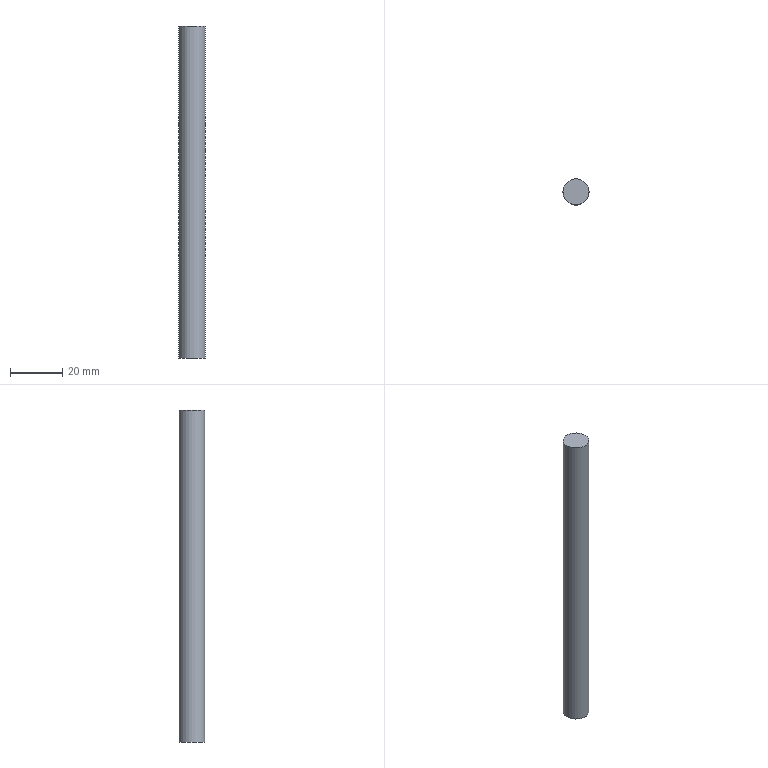Part | STEP file | solid 105 | 1 solid | 3 faces | box 10 x 10 x 127.677 mm | volume 10028 mm3 | plane 2 | cylinder 1 | commonest cylinder face diameters 10 x1